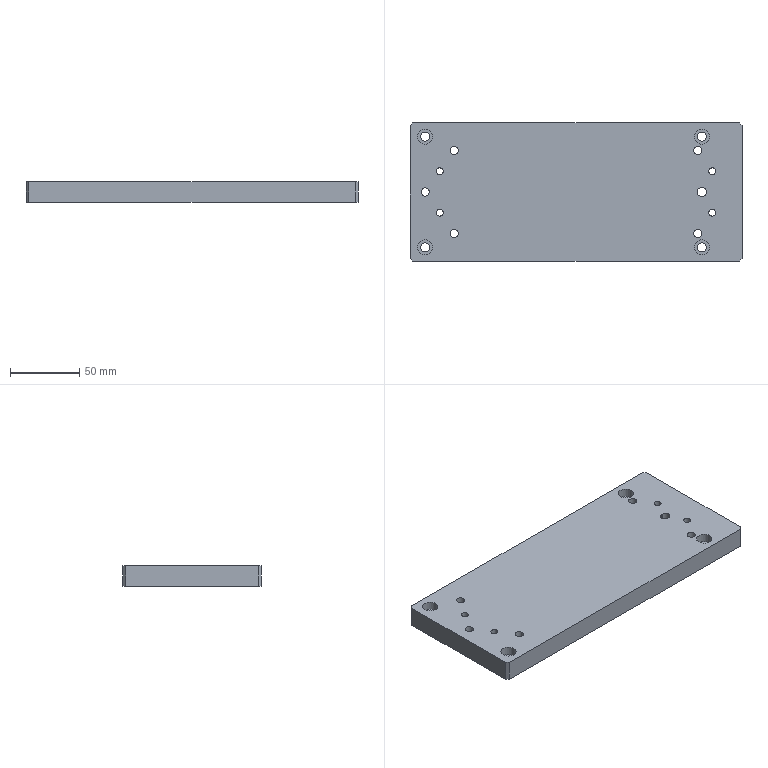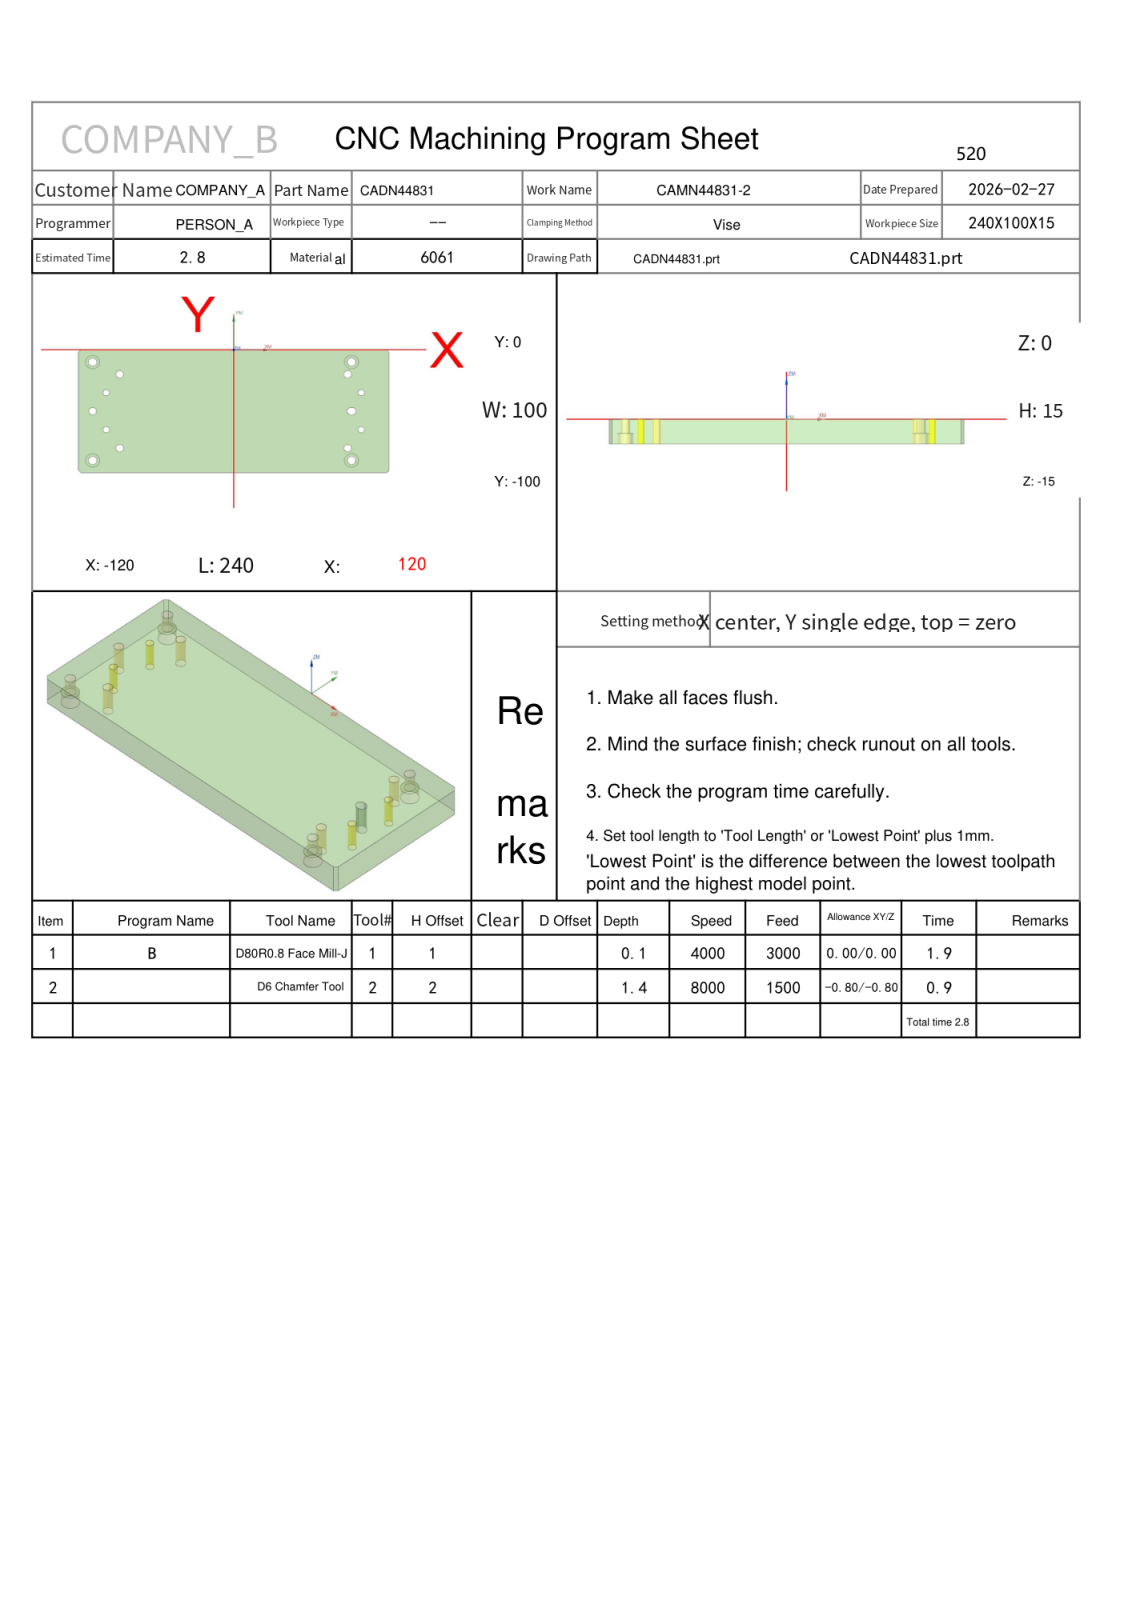NC program | NX | posted by the shop | part box 240 x 100 x 15 mm
Whole program:
%
O0001
(Machine time: 3.18 MIN)
(===Total Tool:2===)
(T1=D80R0.8-FaceMill-J D=80.  R=0.8  D-  H01 Z=0.    )
(T2=D6_ChamferTool   D=6.   R=0.   D-  H02 Z=-1.4  )
G80 G90 G17 G49 G40
G91 G28 Z0
M01
N1 T01 M06
(D80R0.8-FaceMill-J  D=80. R=0.8 H=01 ce=0.10 di=0.10)
G00 G90 G54 X172.097 Y-76.097 M03 S2800
G43 H01 Z50.
M08
Z4.02
G01 Z2.02 F3000.
X160.097
X-152.897
G02 X-160.097 Y-68.897 I0.0 J7.2
G01 Y-39.263
G02 X-152.097 Y-31.263 I8. J0.0
G01 X160.097
X172.097
Z4.02
G00 Y-76.097
Z3.54
G01 Z1.54
X160.097
X-152.897
G02 X-160.097 Y-68.897 I0.0 J7.2
G01 Y-39.263
G02 X-152.097 Y-31.263 I8. J0.0
G01 X160.097
X172.097
Z3.54
G00 Y-76.097
Z3.06
G01 Z1.06
X160.097
X-152.897
G02 X-160.097 Y-68.897 I0.0 J7.2
G01 Y-39.263
G02 X-152.097 Y-31.263 I8. J0.0
G01 X160.097
X172.097
Z3.06
G00 Y-76.097
Z2.58
G01 Z.58
X160.097
X-152.897
G02 X-160.097 Y-68.897 I0.0 J7.2
G01 Y-39.263
G02 X-152.097 Y-31.263 I8. J0.0
G01 X160.097
X172.097
Z2.58
G00 Y-76.097
Z2.1
G01 Z.1
X160.097
X-152.897
G02 X-160.097 Y-68.897 I0.0 J7.2
G01 Y-39.263
G02 X-152.097 Y-31.263 I8. J0.0
G01 X160.097
X172.097
Z2.1
G00 Z50.
G00 G90 X171.999 Y-75.999 M03 S4000
Z50.
Z2.
G01 Z0.0 F1000.
X159.999
X-152.799
G02 X-159.999 Y-68.799 I0.0 J7.2
G01 Y-39.361
G02 X-151.999 Y-31.361 I8. J0.0
G01 X159.999
X171.999
Z2.
G00 Z50.
G91 G28 Z0.0
M05
M09
G91 G28 Z0.0
M01
N2 T02 M06
(D6_ChamferTool  D=6. R=0. H=02 ce=-0.80 di=-0.80)
G00 G90 G54 X-98.732 Y-64.13 M03 S8000
G43 H02 Z50.
M08
Z-.9
G01 Z-1.4 F600.
X-98.9 Y-63.5
G03 X-100.4 Y-65. I0.0 J-1.5
X-98.5 Y-66.9 I1.9 J0.0
X-96.6 Y-65. I0.0 J1.9
X-98.5 Y-63.1 I-1.9 J0.0
X-100.4 Y-65. I0.0 J-1.9
X-98.9 Y-66.5 I1.5 J0.0
G01 X-98.732 Y-65.87
Z-.9
G00 Z50.
Y-34.13
Z-.9
G01 Z-1.4
X-98.9 Y-33.5
G03 X-100.4 Y-35. I0.0 J-1.5
X-98.5 Y-36.9 I1.9 J0.0
X-96.6 Y-35. I0.0 J1.9
X-98.5 Y-33.1 I-1.9 J0.0
X-100.4 Y-35. I0.0 J-1.9
X-98.9 Y-36.5 I1.5 J0.0
G01 X-98.732 Y-35.87
Z-.9
G00 Z50.
X98.268 Y-34.13
Z-.9
G01 Z-1.4
X98.1 Y-33.5
G03 X96.6 Y-35. I0.0 J-1.5
X98.5 Y-36.9 I1.9 J0.0
X100.4 Y-35. I0.0 J1.9
X98.5 Y-33.1 I-1.9 J0.0
X96.6 Y-35. I0.0 J-1.9
X98.1 Y-36.5 I1.5 J0.0
G01 X98.268 Y-35.87
Z-.9
G00 Z50.
Y-64.13
Z-.9
G01 Z-1.4
X98.1 Y-63.5
G03 X96.6 Y-65. I0.0 J-1.5
X98.5 Y-66.9 I1.9 J0.0
X100.4 Y-65. I0.0 J1.9
X98.5 Y-63.1 I-1.9 J0.0
X96.6 Y-65. I0.0 J-1.9
X98.1 Y-66.5 I1.5 J0.0
G01 X98.268 Y-65.87
Z-.9
G00 Z50.
G00 G90 X.386 Y-101.227 M03 S6500
Z50.
Z.172
G01 Z-1.2 F1500.
G03 X.1 Y-101.027 I-1.286 J-1.532
G01 X.054 Y-100.997
X0.0 Y-101.
X-118.
X-118.259 Y-100.966
X-118.5 Y-100.866
X-118.707 Y-100.707
X-120.707 Y-98.707
X-120.866 Y-98.5
X-120.966 Y-98.259
X-121. Y-98.
Y-2.
X-120.966 Y-1.741
X-120.866 Y-1.5
X-120.707 Y-1.293
X-118.707 Y.707
X-118.5 Y.866
X-118.259 Y.966
X-118. Y1.
X118.
X118.259 Y.966
X118.5 Y.866
X118.707 Y.707
X120.707 Y-1.293
X120.866 Y-1.5
X120.966 Y-1.741
X121. Y-2.
Y-98.
X120.966 Y-98.259
X120.866 Y-98.5
X120.707 Y-98.707
X118.707 Y-100.707
X118.5 Y-100.866
X118.259 Y-100.966
X118. Y-101.
X0.0
X-.054 Y-100.997
X-.1 Y-101.027
G03 X-.386 Y-101.227 I1. J-1.732
G01 Z.172
G00 Z10.
X-111.108 Y-89.596
Z.253
G01 Z-1.2
G03 X-111.282 Y-89.898 I1.638 J-1.147
G01 X-111.308 Y-89.946
X-111.3 Y-90.
G03 X-109. Y-92.3 I2.3 J0.0
X-106.7 Y-90. I0.0 J2.3
X-109. Y-87.7 I-2.3 J0.0
X-111.3 Y-90. I0.0 J-2.3
G01 X-111.308 Y-90.054
X-111.282 Y-90.102
G03 X-111.108 Y-90.404 I1.813 J.845
G01 Z.253
G00 Z10.
X-89.808 Y-79.596
Z.257
G01 Z-1.2
G03 X-89.982 Y-79.898 I1.638 J-1.147
G01 X-90.008 Y-79.946
X-90. Y-80.
G03 X-88. Y-82. I2. J0.0
X-86. Y-80. I0.0 J2.
X-88. Y-78. I-2. J0.0
X-89.97 Y-79.653 I0.0 J-2.
G01 X-90. Y-80.
X-90.008 Y-80.054
X-89.982 Y-80.102
G03 X-89.808 Y-80.404 I1.813 J.845
G01 Z.257
G00 Z10.
X-99.815 Y-64.593
Z.284
G01 Z-1.2
G03 X-99.984 Y-64.898 I1.658 J-1.118
G01 X-100.009 Y-64.946
X-100. Y-65.
G03 X-98.5 Y-66.5 I1.5 J0.0
X-97. Y-65. I0.0 J1.5
X-98.5 Y-63.5 I-1.5 J0.0
X-100. Y-65. I0.0 J-1.5
G01 X-100.009 Y-65.054
X-99.984 Y-65.102
G03 X-99.815 Y-65.407 I1.827 J.813
G01 Z.284
G00 Z10.
X-110.808 Y-49.596
Z.257
G01 Z-1.2
G03 X-110.982 Y-49.898 I1.638 J-1.147
G01 X-111.008 Y-49.946
X-111. Y-50.
G03 X-109. Y-52. I2. J0.0
X-107. Y-50. I0.0 J2.
X-109. Y-48. I-2. J0.0
X-110.97 Y-49.653 I0.0 J-2.
G01 X-111. Y-50.
X-111.008 Y-50.054
X-110.982 Y-50.102
G03 X-110.808 Y-50.404 I1.813 J.845
G01 Z.257
G00 Z10.
X-99.815 Y-34.593
Z.284
G01 Z-1.2
G03 X-99.984 Y-34.898 I1.658 J-1.118
G01 X-100.009 Y-34.946
X-100. Y-35.
G03 X-98.5 Y-36.5 I1.5 J0.0
X-97. Y-35. I0.0 J1.5
X-98.5 Y-33.5 I-1.5 J0.0
X-100. Y-35. I0.0 J-1.5
G01 X-100.009 Y-35.054
X-99.984 Y-35.102
G03 X-99.815 Y-35.407 I1.827 J.813
G01 Z.284
G00 Z10.
X-111.108 Y-9.596
Z.253
G01 Z-1.2
G03 X-111.282 Y-9.898 I1.638 J-1.147
G01 X-111.308 Y-9.946
X-111.3 Y-10.
G03 X-109. Y-12.3 I2.3 J0.0
X-106.7 Y-10. I0.0 J2.3
X-109. Y-7.7 I-2.3 J0.0
X-111.3 Y-10. I0.0 J-2.3
G01 X-111.308 Y-10.054
X-111.282 Y-10.102
G03 X-111.108 Y-10.404 I1.813 J.845
G01 Z.253
G00 Z10.
X-89.808 Y-19.596
Z.257
G01 Z-1.2
G03 X-89.982 Y-19.898 I1.638 J-1.147
G01 X-90.008 Y-19.946
X-90. Y-20.
G03 X-88. Y-22. I2. J0.0
X-86. Y-20. I0.0 J2.
X-88. Y-18. I-2. J0.0
X-89.97 Y-19.653 I0.0 J-2.
G01 X-90. Y-20.
X-90.008 Y-20.054
X-89.982 Y-20.102
G03 X-89.808 Y-20.404 I1.813 J.845
G01 Z.257
G00 Z10.
X88.892 Y-9.596
Z.253
G01 Z-1.2
G03 X88.718 Y-9.898 I1.638 J-1.147
G01 X88.692 Y-9.946
X88.7 Y-10.
G03 X91. Y-12.3 I2.3 J0.0
X93.3 Y-10. I0.0 J2.3
X91. Y-7.7 I-2.3 J0.0
X88.7 Y-10. I0.0 J-2.3
G01 X88.692 Y-10.054
X88.718 Y-10.102
G03 X88.892 Y-10.404 I1.813 J.845
G01 Z.253
G00 Z2.55
X86.192 Y-19.596
Z.257
G01 Z-1.2
G03 X86.018 Y-19.898 I1.638 J-1.147
G01 X85.992 Y-19.946
X86. Y-20.
G03 X88. Y-22. I2. J0.0
X90. Y-20. I0.0 J2.
X88. Y-18. I-2. J0.0
X86.03 Y-19.653 I0.0 J-2.
G01 X86. Y-20.
X85.992 Y-20.054
X86.018 Y-20.102
G03 X86.192 Y-20.404 I1.813 J.845
G01 Z.257
G00 Z10.
X97.185 Y-34.593
Z.284
G01 Z-1.2
G03 X97.016 Y-34.898 I1.658 J-1.118
G01 X96.991 Y-34.946
X97. Y-35.
G03 X98.5 Y-36.5 I1.5 J0.0
X100. Y-35. I0.0 J1.5
X98.5 Y-33.5 I-1.5 J0.0
X97. Y-35. I0.0 J-1.5
G01 X96.991 Y-35.054
X97.016 Y-35.102
G03 X97.185 Y-35.407 I1.827 J.813
G01 Z.284
G00 Z10.
X90.614 Y-51.773
Z.172
G01 Z-1.2
G03 X90.9 Y-51.973 I1.286 J1.532
G01 X90.946 Y-52.003
X91. Y-52.
X91.5
G03 X93.5 Y-50. I0.0 J2.
X91.5 Y-48. I-2. J0.0
G01 X90.5
G03 X88.5 Y-50. I0.0 J-2.
X90.5 Y-52. I2. J0.0
G01 X91.
X91.054 Y-52.003
X91.1 Y-51.973
G03 X91.386 Y-51.773 I-1. J1.732
G01 Z.172
G00 Z10.
X97.185 Y-64.593
Z.284
G01 Z-1.2
G03 X97.016 Y-64.898 I1.658 J-1.118
G01 X96.991 Y-64.946
X97. Y-65.
G03 X98.5 Y-66.5 I1.5 J0.0
X100. Y-65. I0.0 J1.5
X98.5 Y-63.5 I-1.5 J0.0
X97. Y-65. I0.0 J-1.5
G01 X96.991 Y-65.054
X97.016 Y-65.102
G03 X97.185 Y-65.407 I1.827 J.813
G01 Z.284
G00 Z10.
X86.192 Y-79.596
Z.257
G01 Z-1.2
G03 X86.018 Y-79.898 I1.638 J-1.147
G01 X85.992 Y-79.946
X86. Y-80.
G03 X88. Y-82. I2. J0.0
X90. Y-80. I0.0 J2.
X88. Y-78. I-2. J0.0
X86.03 Y-79.653 I0.0 J-2.
G01 X86. Y-80.
X85.992 Y-80.054
X86.018 Y-80.102
G03 X86.192 Y-80.404 I1.813 J.845
G01 Z.257
G00 Z2.55
X88.892 Y-89.596
Z.253
G01 Z-1.2
G03 X88.718 Y-89.898 I1.638 J-1.147
G01 X88.692 Y-89.946
X88.7 Y-90.
G03 X91. Y-92.3 I2.3 J0.0
X93.3 Y-90. I0.0 J2.3
X91. Y-87.7 I-2.3 J0.0
X88.7 Y-90. I0.0 J-2.3
G01 X88.692 Y-90.054
X88.718 Y-90.102
G03 X88.892 Y-90.404 I1.813 J.845
G01 Z.253
G00 Z50.
M05
M09
G91 G28 Z0.0
G91 G28 Y0.0
M30
%